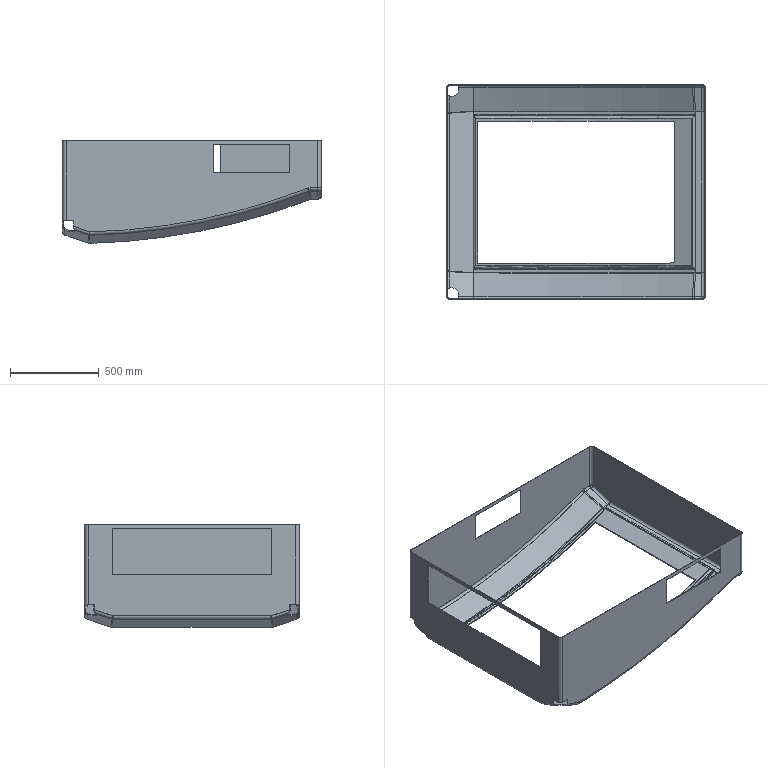Part | SolidWorks | features ICE 7, Chamfer 3, Fillet 2, MoveFace 2, Shell 1 | 1 solid | 158 faces | box 1460 x 1210 x 578.799 mm | volume 14635130 mm3 | cylinder 47 | plane 43 | spline 32 | torus 16 | sphere 16 | cone 4 | commonest cylinder face diameters 30 x18 40 x15 80 x4 20 x3 7422 x2 7432 x2